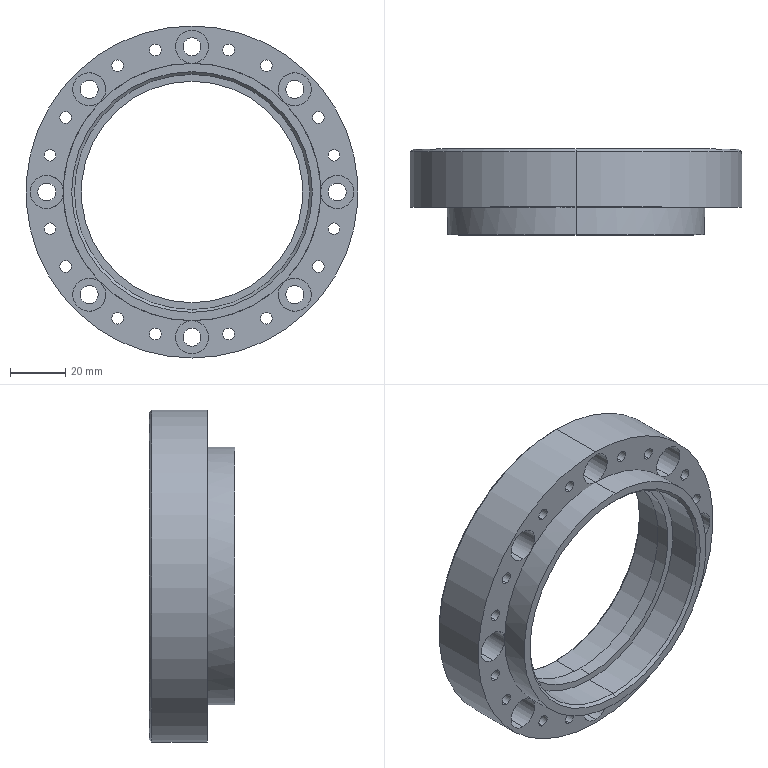Part | SolidWorks | features CirPattern 3, Chamfer 2, Cut 2, HoleWzd 2, ICE 2, Extrusion 1 | 1 solid | 93 faces | box 120 x 31 x 120 mm | volume 115684 mm3 | cylinder 74 | plane 13 | cone 6 | commonest cylinder face diameters 4.2 x32 6.5 x16 12 x16 85 x4 80 x2 93 x2